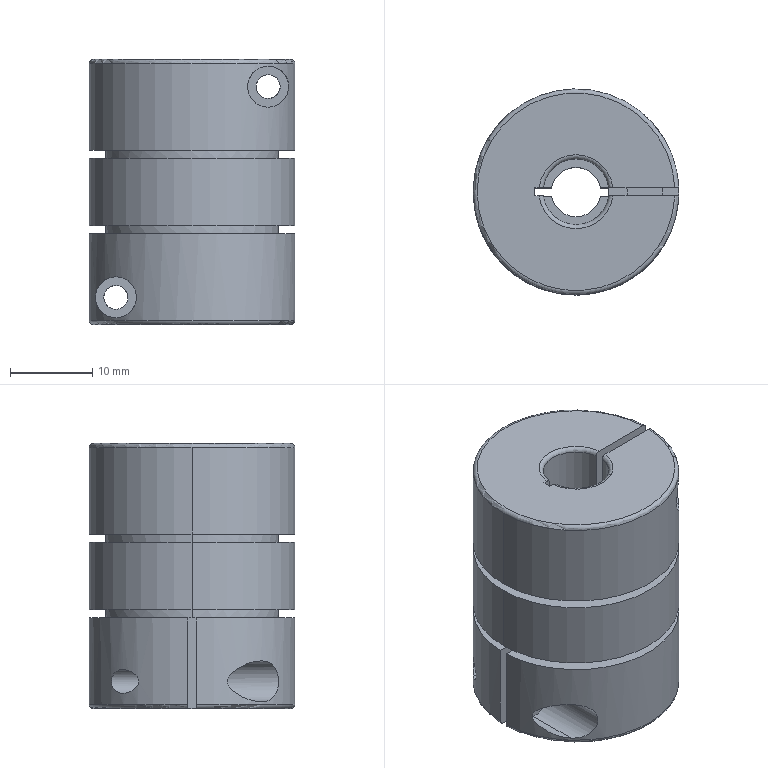Part | STEP file | XHW-25C-6×8 | 1 solid | 56 faces | box 25 x 25 x 32.2 mm | volume 12804 mm3 | cylinder 27 | plane 22 | torus 7 | commonest cylinder face diameters 2.9 x8 25 x5 5 x4 21 x4 6 x2 8 x2